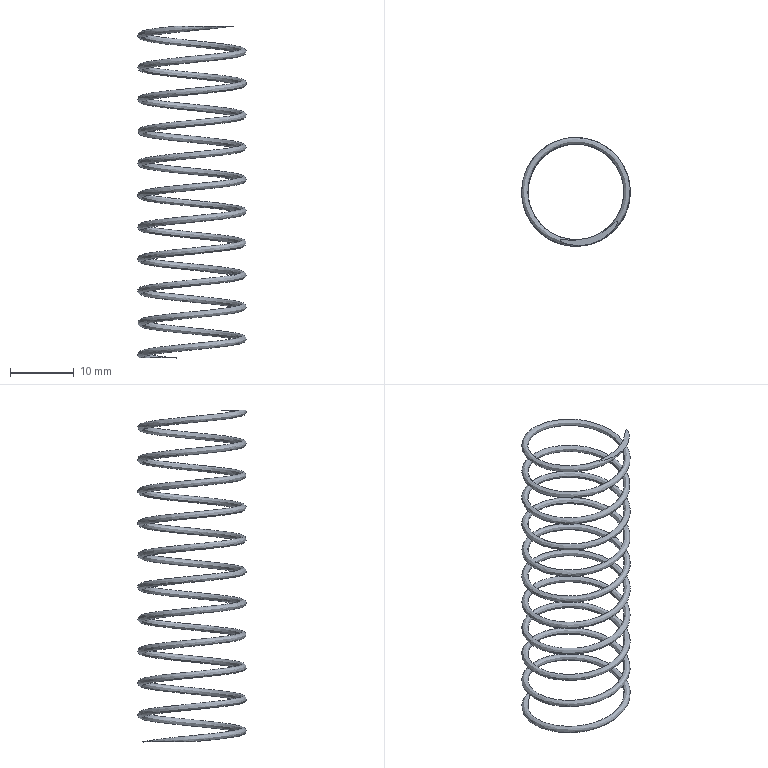Part | NX | features solid 2 | 1 solid | 3 faces | box 17.001 x 17.001 x 52 mm | volume 425.076 mm3 | plane 2 | spline 1